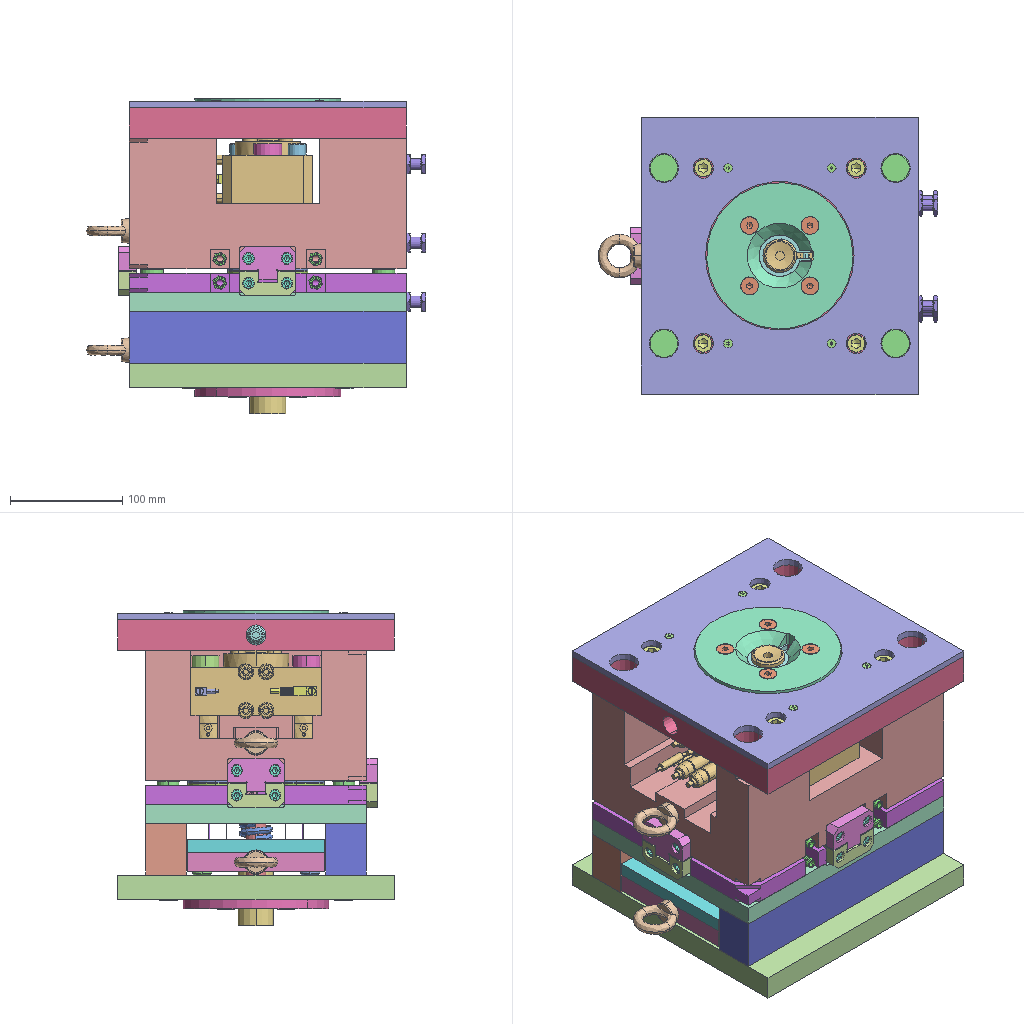Assembly | STEP file | 66 different items | 137 placed | box 302 x 246 x 280 mm
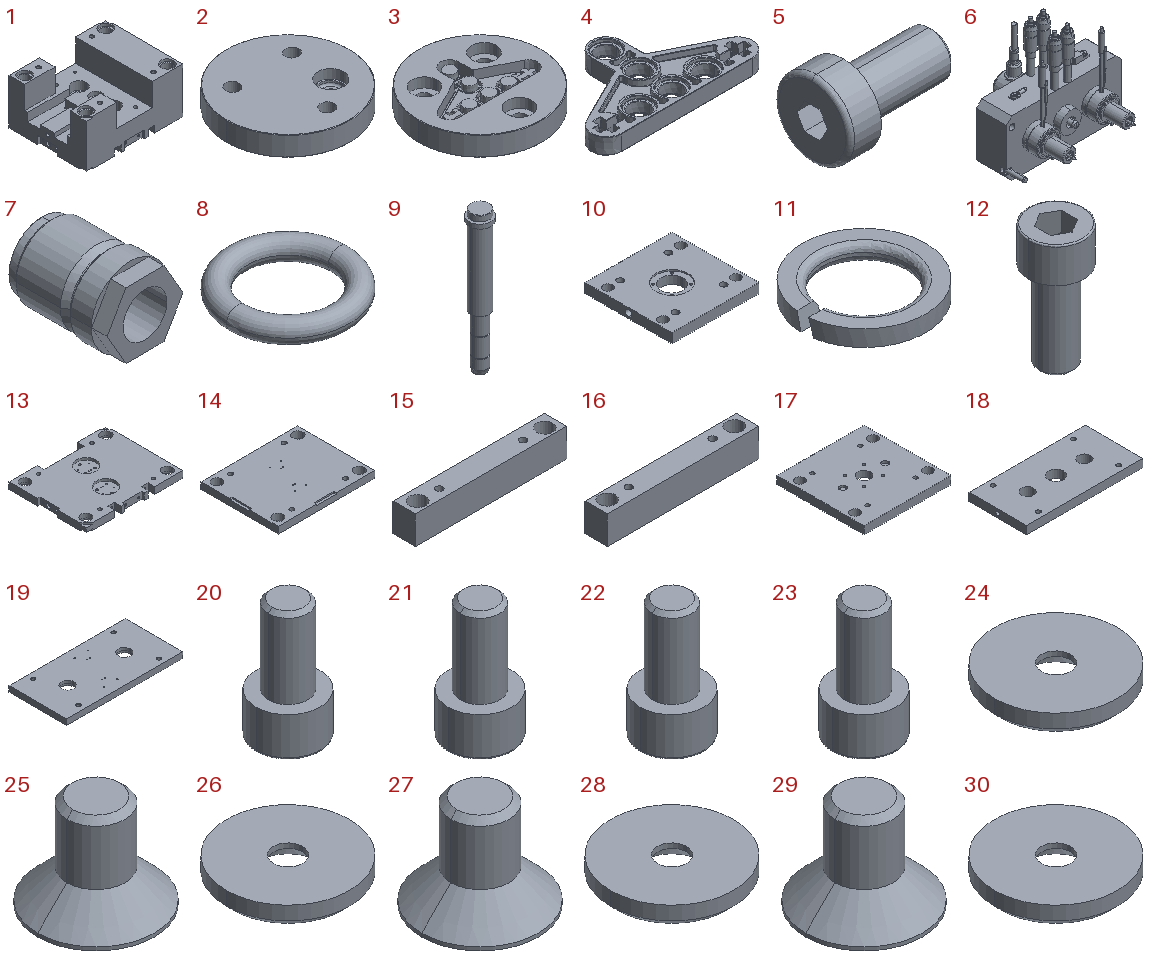Parts list (item | name | quantity | parent item | size | volume):
1 | 2 | x1 | - | 246 x 196 x 116 mm | 3430597 mm3
2 | Cavity | x2 | in Injection system, Forming insert | 50 x 50 x 9.963 mm | 14384 mm3
3 | Core | x2 | in Injection system, Forming insert | 50 x 50 x 8 mm | 13150 mm3
4 | Moulded part | x2 | in Injection system, Forming insert | 39.381 x 23.386 x 3.923 mm | 972.135 mm3
5 | socket head thin cap screw_din_DIN 7984 - M5 x 10 --- 7.6N | x12 | in Injection system, Forming insert | 13.5 x 8.5 x 8.5 mm | 369.151 mm3
6 | COMPANY_A | x1 | in Injection system | - | -
7 | export_nozzle | x2 | in Injection system | 10.5 x 14.1 x 10.5 mm | 682.036 mm3
8 | o-rings_am_J515160x0061H | x2 | in Injection system | 9.3 x 9.3 x 1.6 mm | 48.637 mm3
9 | 38 | x4 | - | 31 x 31 x 200 mm | 90446 mm3
10 | 1 | x1 | - | 246 x 246 x 27 mm | 1437591 mm3
11 | 44 | x4 | - | 15.198 x 15.2 x 2 mm | 183.52 mm3
12 | 45 | x4 | - | 16 x 16 x 35 mm | 3597 mm3
13 | 3 | x1 | in FCPK-196x246_PKA_PKA01-27-1.1730_PKA03-116-1.1730_PKA03-17-1.1730_YES_PKA04-17-1.1730_PKA05-46-1.1730_PKA06-12-1.1730_PKA07-17-1.1730_PKA11-22-1.1730_SLE-75-1.7131_TPE-1.7131 | 246 x 196 x 17 mm | 676741 mm3
14 | 4 | x1 | in FCPK-196x246_PKA_PKA01-27-1.1730_PKA03-116-1.1730_PKA03-17-1.1730_YES_PKA04-17-1.1730_PKA05-46-1.1730_PKA06-12-1.1730_PKA07-17-1.1730_PKA11-22-1.1730_SLE-75-1.7131_TPE-1.7131 | 246 x 196 x 17 mm | 768629 mm3
15 | 5 | x1 | in FCPK-196x246_PKA_PKA01-27-1.1730_PKA03-116-1.1730_PKA03-17-1.1730_YES_PKA04-17-1.1730_PKA05-46-1.1730_PKA06-12-1.1730_PKA07-17-1.1730_PKA11-22-1.1730_SLE-75-1.7131_TPE-1.7131 | 246 x 36 x 46 mm | 349787 mm3
16 | 6 | x1 | in FCPK-196x246_PKA_PKA01-27-1.1730_PKA03-116-1.1730_PKA03-17-1.1730_YES_PKA04-17-1.1730_PKA05-46-1.1730_PKA06-12-1.1730_PKA07-17-1.1730_PKA11-22-1.1730_SLE-75-1.7131_TPE-1.7131 | 246 x 36 x 46 mm | 349787 mm3
17 | 7 | x1 | in FCPK-196x246_PKA_PKA01-27-1.1730_PKA03-116-1.1730_PKA03-17-1.1730_YES_PKA04-17-1.1730_PKA05-46-1.1730_PKA06-12-1.1730_PKA07-17-1.1730_PKA11-22-1.1730_SLE-75-1.7131_TPE-1.7131 | 246 x 246 x 22 mm | 1219815 mm3
18 | 8 | x1 | in FCPK-196x246_PKA_PKA01-27-1.1730_PKA03-116-1.1730_PKA03-17-1.1730_YES_PKA04-17-1.1730_PKA05-46-1.1730_PKA06-12-1.1730_PKA07-17-1.1730_PKA11-22-1.1730_SLE-75-1.7131_TPE-1.7131 | 246 x 122 x 17 mm | 467682 mm3
19 | 9 | x1 | in FCPK-196x246_PKA_PKA01-27-1.1730_PKA03-116-1.1730_PKA03-17-1.1730_YES_PKA04-17-1.1730_PKA05-46-1.1730_PKA06-12-1.1730_PKA07-17-1.1730_PKA11-22-1.1730_SLE-75-1.7131_TPE-1.7131 | 246 x 122 x 12 mm | 330274 mm3
20 | 10 | x1 | in FCPK-196x246_PKA_PKA01-27-1.1730_PKA03-116-1.1730_PKA03-17-1.1730_YES_PKA04-17-1.1730_PKA05-46-1.1730_PKA06-12-1.1730_PKA07-17-1.1730_PKA11-22-1.1730_SLE-75-1.7131_TPE-1.7131 | 13 x 13 x 24 mm | 1690 mm3
21 | 11 | x1 | in FCPK-196x246_PKA_PKA01-27-1.1730_PKA03-116-1.1730_PKA03-17-1.1730_YES_PKA04-17-1.1730_PKA05-46-1.1730_PKA06-12-1.1730_PKA07-17-1.1730_PKA11-22-1.1730_SLE-75-1.7131_TPE-1.7131 | 13 x 13 x 24 mm | 1690 mm3
22 | 12 | x1 | in FCPK-196x246_PKA_PKA01-27-1.1730_PKA03-116-1.1730_PKA03-17-1.1730_YES_PKA04-17-1.1730_PKA05-46-1.1730_PKA06-12-1.1730_PKA07-17-1.1730_PKA11-22-1.1730_SLE-75-1.7131_TPE-1.7131 | 13 x 13 x 24 mm | 1690 mm3
23 | 13 | x1 | in FCPK-196x246_PKA_PKA01-27-1.1730_PKA03-116-1.1730_PKA03-17-1.1730_YES_PKA04-17-1.1730_PKA05-46-1.1730_PKA06-12-1.1730_PKA07-17-1.1730_PKA11-22-1.1730_SLE-75-1.7131_TPE-1.7131 | 13 x 13 x 24 mm | 1690 mm3
24 | 14 | x1 | in FCPK-196x246_PKA_PKA01-27-1.1730_PKA03-116-1.1730_PKA03-17-1.1730_YES_PKA04-17-1.1730_PKA05-46-1.1730_PKA06-12-1.1730_PKA07-17-1.1730_PKA11-22-1.1730_SLE-75-1.7131_TPE-1.7131 | 18 x 18 x 3 mm | 644.142 mm3
25 | 15 | x1 | in FCPK-196x246_PKA_PKA01-27-1.1730_PKA03-116-1.1730_PKA03-17-1.1730_YES_PKA04-17-1.1730_PKA05-46-1.1730_PKA06-12-1.1730_PKA07-17-1.1730_PKA11-22-1.1730_SLE-75-1.7131_TPE-1.7131 | 10 x 10 x 8 mm | 218.465 mm3
26 | 16 | x1 | in FCPK-196x246_PKA_PKA01-27-1.1730_PKA03-116-1.1730_PKA03-17-1.1730_YES_PKA04-17-1.1730_PKA05-46-1.1730_PKA06-12-1.1730_PKA07-17-1.1730_PKA11-22-1.1730_SLE-75-1.7131_TPE-1.7131 | 18 x 18 x 3 mm | 644.142 mm3
27 | 17 | x1 | in FCPK-196x246_PKA_PKA01-27-1.1730_PKA03-116-1.1730_PKA03-17-1.1730_YES_PKA04-17-1.1730_PKA05-46-1.1730_PKA06-12-1.1730_PKA07-17-1.1730_PKA11-22-1.1730_SLE-75-1.7131_TPE-1.7131 | 10 x 10 x 8 mm | 218.465 mm3
28 | 18 | x1 | in FCPK-196x246_PKA_PKA01-27-1.1730_PKA03-116-1.1730_PKA03-17-1.1730_YES_PKA04-17-1.1730_PKA05-46-1.1730_PKA06-12-1.1730_PKA07-17-1.1730_PKA11-22-1.1730_SLE-75-1.7131_TPE-1.7131 | 18 x 18 x 3 mm | 644.142 mm3
29 | 19 | x1 | in FCPK-196x246_PKA_PKA01-27-1.1730_PKA03-116-1.1730_PKA03-17-1.1730_YES_PKA04-17-1.1730_PKA05-46-1.1730_PKA06-12-1.1730_PKA07-17-1.1730_PKA11-22-1.1730_SLE-75-1.7131_TPE-1.7131 | 10 x 10 x 8 mm | 218.465 mm3
30 | 20 | x1 | in FCPK-196x246_PKA_PKA01-27-1.1730_PKA03-116-1.1730_PKA03-17-1.1730_YES_PKA04-17-1.1730_PKA05-46-1.1730_PKA06-12-1.1730_PKA07-17-1.1730_PKA11-22-1.1730_SLE-75-1.7131_TPE-1.7131 | 18 x 18 x 3 mm | 644.142 mm3
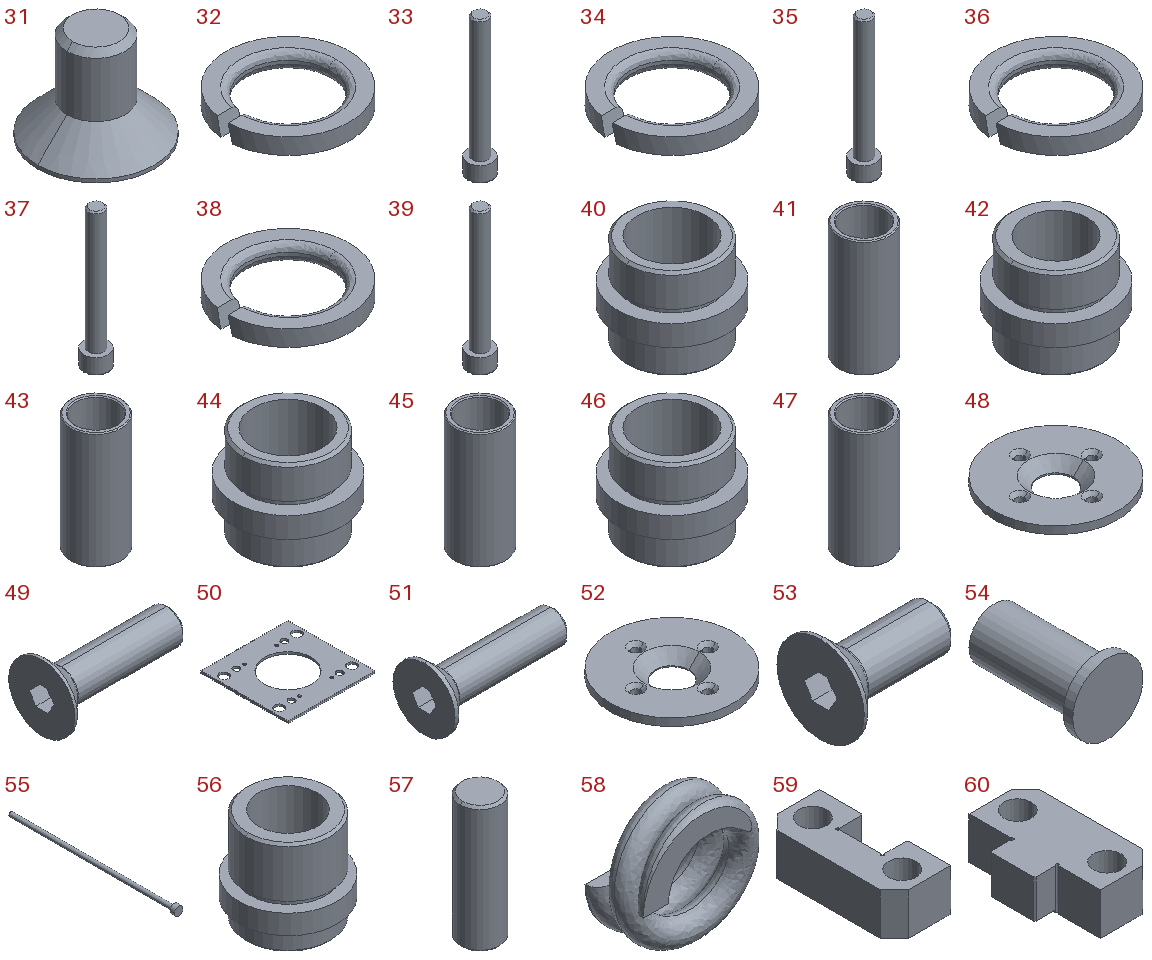31 | 21 | x1 | in FCPK-196x246_PKA_PKA01-27-1.1730_PKA03-116-1.1730_PKA03-17-1.1730_YES_PKA04-17-1.1730_PKA05-46-1.1730_PKA06-12-1.1730_PKA07-17-1.1730_PKA11-22-1.1730_SLE-75-1.7131_TPE-1.7131 | 10 x 10 x 8 mm | 218.465 mm3
32 | 22 | x1 | in FCPK-196x246_PKA_PKA01-27-1.1730_PKA03-116-1.1730_PKA03-17-1.1730_YES_PKA04-17-1.1730_PKA05-46-1.1730_PKA06-12-1.1730_PKA07-17-1.1730_PKA11-22-1.1730_SLE-75-1.7131_TPE-1.7131 | 15.198 x 15.2 x 2 mm | 183.545 mm3
33 | 23 | x1 | in FCPK-196x246_PKA_PKA01-27-1.1730_PKA03-116-1.1730_PKA03-17-1.1730_YES_PKA04-17-1.1730_PKA05-46-1.1730_PKA06-12-1.1730_PKA07-17-1.1730_PKA11-22-1.1730_SLE-75-1.7131_TPE-1.7131 | 16 x 16 x 90 mm | 7916 mm3
34 | 24 | x1 | in FCPK-196x246_PKA_PKA01-27-1.1730_PKA03-116-1.1730_PKA03-17-1.1730_YES_PKA04-17-1.1730_PKA05-46-1.1730_PKA06-12-1.1730_PKA07-17-1.1730_PKA11-22-1.1730_SLE-75-1.7131_TPE-1.7131 | 15.198 x 15.2 x 2 mm | 183.545 mm3
35 | 25 | x1 | in FCPK-196x246_PKA_PKA01-27-1.1730_PKA03-116-1.1730_PKA03-17-1.1730_YES_PKA04-17-1.1730_PKA05-46-1.1730_PKA06-12-1.1730_PKA07-17-1.1730_PKA11-22-1.1730_SLE-75-1.7131_TPE-1.7131 | 16 x 16 x 90 mm | 7916 mm3
36 | 26 | x1 | in FCPK-196x246_PKA_PKA01-27-1.1730_PKA03-116-1.1730_PKA03-17-1.1730_YES_PKA04-17-1.1730_PKA05-46-1.1730_PKA06-12-1.1730_PKA07-17-1.1730_PKA11-22-1.1730_SLE-75-1.7131_TPE-1.7131 | 15.198 x 15.2 x 2 mm | 183.545 mm3
37 | 27 | x1 | in FCPK-196x246_PKA_PKA01-27-1.1730_PKA03-116-1.1730_PKA03-17-1.1730_YES_PKA04-17-1.1730_PKA05-46-1.1730_PKA06-12-1.1730_PKA07-17-1.1730_PKA11-22-1.1730_SLE-75-1.7131_TPE-1.7131 | 16 x 16 x 90 mm | 7916 mm3
38 | 28 | x1 | in FCPK-196x246_PKA_PKA01-27-1.1730_PKA03-116-1.1730_PKA03-17-1.1730_YES_PKA04-17-1.1730_PKA05-46-1.1730_PKA06-12-1.1730_PKA07-17-1.1730_PKA11-22-1.1730_SLE-75-1.7131_TPE-1.7131 | 15.198 x 15.2 x 2 mm | 183.545 mm3
39 | 29 | x1 | in FCPK-196x246_PKA_PKA01-27-1.1730_PKA03-116-1.1730_PKA03-17-1.1730_YES_PKA04-17-1.1730_PKA05-46-1.1730_PKA06-12-1.1730_PKA07-17-1.1730_PKA11-22-1.1730_SLE-75-1.7131_TPE-1.7131 | 16 x 16 x 90 mm | 7916 mm3
40 | 30 | x1 | in FCPK-196x246_PKA_PKA01-27-1.1730_PKA03-116-1.1730_PKA03-17-1.1730_YES_PKA04-17-1.1730_PKA05-46-1.1730_PKA06-12-1.1730_PKA07-17-1.1730_PKA11-22-1.1730_SLE-75-1.7131_TPE-1.7131 | 31 x 31 x 26 mm | 6604 mm3
41 | 31 | x1 | in FCPK-196x246_PKA_PKA01-27-1.1730_PKA03-116-1.1730_PKA03-17-1.1730_YES_PKA04-17-1.1730_PKA05-46-1.1730_PKA06-12-1.1730_PKA07-17-1.1730_PKA11-22-1.1730_SLE-75-1.7131_TPE-1.7131 | 26 x 26 x 60 mm | 14379 mm3
42 | 32 | x1 | in FCPK-196x246_PKA_PKA01-27-1.1730_PKA03-116-1.1730_PKA03-17-1.1730_YES_PKA04-17-1.1730_PKA05-46-1.1730_PKA06-12-1.1730_PKA07-17-1.1730_PKA11-22-1.1730_SLE-75-1.7131_TPE-1.7131 | 31 x 31 x 26 mm | 8159 mm3
43 | 33 | x1 | in FCPK-196x246_PKA_PKA01-27-1.1730_PKA03-116-1.1730_PKA03-17-1.1730_YES_PKA04-17-1.1730_PKA05-46-1.1730_PKA06-12-1.1730_PKA07-17-1.1730_PKA11-22-1.1730_SLE-75-1.7131_TPE-1.7131 | 26 x 26 x 60 mm | 14379 mm3
44 | 34 | x1 | in FCPK-196x246_PKA_PKA01-27-1.1730_PKA03-116-1.1730_PKA03-17-1.1730_YES_PKA04-17-1.1730_PKA05-46-1.1730_PKA06-12-1.1730_PKA07-17-1.1730_PKA11-22-1.1730_SLE-75-1.7131_TPE-1.7131 | 31 x 31 x 26 mm | 6604 mm3
45 | 35 | x1 | in FCPK-196x246_PKA_PKA01-27-1.1730_PKA03-116-1.1730_PKA03-17-1.1730_YES_PKA04-17-1.1730_PKA05-46-1.1730_PKA06-12-1.1730_PKA07-17-1.1730_PKA11-22-1.1730_SLE-75-1.7131_TPE-1.7131 | 26 x 26 x 60 mm | 14379 mm3
46 | 36 | x1 | in FCPK-196x246_PKA_PKA01-27-1.1730_PKA03-116-1.1730_PKA03-17-1.1730_YES_PKA04-17-1.1730_PKA05-46-1.1730_PKA06-12-1.1730_PKA07-17-1.1730_PKA11-22-1.1730_SLE-75-1.7131_TPE-1.7131 | 31 x 31 x 26 mm | 6604 mm3
47 | 37 | x1 | in FCPK-196x246_PKA_PKA01-27-1.1730_PKA03-116-1.1730_PKA03-17-1.1730_YES_PKA04-17-1.1730_PKA05-46-1.1730_PKA06-12-1.1730_PKA07-17-1.1730_PKA11-22-1.1730_SLE-75-1.7131_TPE-1.7131 | 26 x 26 x 60 mm | 14379 mm3
48 | PCA-130120 | x1 | - | 130 x 130 x 12 mm | 106365 mm3
49 | socket countersunk head screw_din_DIN 7991 - M8 x 30 --- 21.8N | x4 | - | 30 x 15.57 x 15.57 mm | 1740 mm3
50 | Insulating plate | x2 | - | 246 x 246 x 6 mm | 261647 mm3
51 | socket countersunk head screw_din_DIN 7991 - M4 x 16 --- 11.6N | x4 | - | 16 x 7.64 x 7.64 mm | 232.169 mm3
52 | PCA-130120 unmachined | x1 | - | 130 x 130 x 12 mm | 107256 mm3
53 | socket countersunk head screw_din_DIN 7991 - M8 x 20 --- 11.8N | x4 | - | 20 x 15.57 x 15.57 mm | 1237 mm3
54 | Main ejector | x1 | - | 44 x 71 x 44 mm | 61399 mm3
55 | ejector | x8 | - | 3 x 58.08 x 3 mm | 97.701 mm3
56 | TBW-1812 | x2 | - | 30 x 30 x 29 mm | 8727 mm3
57 | Ejector guide | x2 | - | 18 x 18 x 58 mm | 14705 mm3
58 | Ejector spring 14 | x2 | - | 30 x 14 x 30 mm | 3867 mm3
59 | 1_1 | x2 | in MS50-050 | 21.5 x 50 x 16 mm | 12210 mm3
60 | 2_1 | x2 | in MS50-050 | 30 x 50 x 16 mm | 16891 mm3
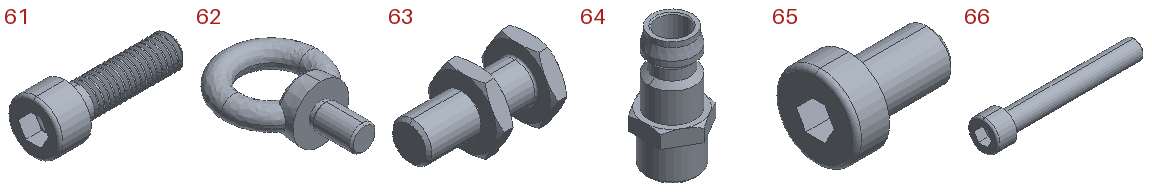61 | socket head cap screw 4762_din_ISO 4762 M6 x 20 --- 20S | x8 | in MS50-050 | 26 x 10 x 10 mm | 892.13 mm3
62 | Part 65 | x2 | - | 38.75 x 55.625 x 21.875 mm | 8627 mm3
63 | Part 66 | x6 | - | 31.25 x 19.486 x 16.875 mm | 3681 mm3
64 | KH-060 ENM 10 | x8 | - | 11 x 12.702 x 24 mm | 962.573 mm3
65 | socket head thin cap screw_din_DIN 7984 - M6 x 10 --- 7N | x4 | - | 14 x 10 x 10 mm | 545.673 mm3
66 | socket head cap screw fine_din_DIN 912 M10x1 x 70 --- 32N | x2 | - | 80 x 16 x 16 mm | 7176 mm3
Placements (level | parent | child | x y z in mm | rotation matrix by rows):
1 | subassembly 2 | 2 | -0.0 -0.0 -0.0 | 1 0 0 0 1 0 0 0 1
1 | subassembly 2 | Injection system | 52.614 -35.372 53.014 | 1 0 0 0 1 0 0 0 1
2 | Injection system | Cavity | -79.114 -4.052 45.024 | 1 0 0 0 1 0 0 0 1
2 | Injection system | Core | -79.114 -4.052 45.024 | 1 0 0 0 1 0 0 0 1
2 | Injection system | Moulded part | -79.114 -4.052 45.024 | 1 0 0 0 1 0 0 0 1
2 | Injection system | socket head thin cap screw_din_DIN 7984 - M5 x 10 --- 7.6N | -51.122 10.1 46.586 | 0 0 1 0 1 0 -1 0 0
2 | Injection system | socket head thin cap screw_din_DIN 7984 - M5 x 10 --- 7.6N | -63.214 -16.378 47.386 | 0 -0.383 -0.9237 0 0.9237 -0.383 1 0 0
2 | Injection system | socket head thin cap screw_din_DIN 7984 - M5 x 10 --- 7.6N | -63.214 -16.378 46.586 | 0 0 1 0 1 0 -1 0 0
2 | Injection system | socket head thin cap screw_din_DIN 7984 - M5 x 10 --- 7.6N | -75.306 10.1 46.586 | 0 0 1 0 1 0 -1 0 0
2 | Injection system | socket head thin cap screw_din_DIN 7984 - M5 x 10 --- 7.6N | -75.306 10.1 47.386 | 0 -0.383 -0.9237 0 0.9237 -0.383 1 0 0
2 | Injection system | socket head thin cap screw_din_DIN 7984 - M5 x 10 --- 7.6N | -51.122 10.1 47.386 | 0 -0.383 -0.9237 0 0.9237 -0.383 1 0 0
2 | Injection system | COMPANY_A | -52.614 35.372 149.986 | 0 0 -1 -1 0 0 0 1 0
2 | Injection system | Forming insert | -105.228 70.745 0.0 | -1 0 0 0 -1 0 0 0 1
3 | Forming insert | Cavity | -79.114 -4.052 45.024 | 1 0 0 0 1 0 0 0 1
3 | Forming insert | Core | -79.114 -4.052 45.024 | 1 0 0 0 1 0 0 0 1
3 | Forming insert | Moulded part | -79.114 -4.052 45.024 | 1 0 0 0 1 0 0 0 1
3 | Forming insert | socket head thin cap screw_din_DIN 7984 - M5 x 10 --- 7.6N | -51.122 10.1 46.586 | 0 0 1 0 1 0 -1 0 0
3 | Forming insert | socket head thin cap screw_din_DIN 7984 - M5 x 10 --- 7.6N | -63.214 -16.378 47.386 | 0 -0.383 -0.9237 0 0.9237 -0.383 1 0 0
3 | Forming insert | socket head thin cap screw_din_DIN 7984 - M5 x 10 --- 7.6N | -63.214 -16.378 46.586 | 0 0 1 0 1 0 -1 0 0
3 | Forming insert | socket head thin cap screw_din_DIN 7984 - M5 x 10 --- 7.6N | -75.306 10.1 46.586 | 0 0 1 0 1 0 -1 0 0
3 | Forming insert | socket head thin cap screw_din_DIN 7984 - M5 x 10 --- 7.6N | -75.306 10.1 47.386 | 0 -0.383 -0.9237 0 0.9237 -0.383 1 0 0
3 | Forming insert | socket head thin cap screw_din_DIN 7984 - M5 x 10 --- 7.6N | -51.122 10.1 47.386 | 0 -0.383 -0.9237 0 0.9237 -0.383 1 0 0
2 | Injection system | export_nozzle | -10.114 -7.128 146.986 | 1 0 0 0 0 -1 0 1 0
2 | Injection system | export_nozzle | -10.114 77.872 146.986 | 1 0 0 0 0 -1 0 1 0
2 | Injection system | o-rings_am_J515160x0061H | -52.614 77.872 50.486 | 1 0 0 0 1 0 0 0 1
2 | Injection system | o-rings_am_J515160x0061H | -52.614 -7.128 50.486 | -0.9237 -0.383 0 -0.383 0.9237 0 0 0 -1
1 | subassembly 2 | 38 | -0.0 -156.0 -0.0 | 1 0 0 0 1 0 0 0 1
1 | subassembly 2 | 1 | -0.0 -0.0 -0.0 | 1 0 0 0 1 0 0 0 1
1 | subassembly 2 | 44 | -136.0 -156.0 -0.0 | 1 0 0 0 1 0 0 0 1
1 | subassembly 2 | 45 | -136.0 -156.0 0.0 | 1 0 0 0 1 0 0 0 1
1 | subassembly 2 | 38 | -206.0 156.0 -0.0 | -1 0 0 0 -1 0 0 0 1
1 | subassembly 2 | 45 | -0.0 156.0 0.0 | -1 0 0 0 -1 0 0 0 1
1 | subassembly 2 | 44 | -136.0 -0.0 -0.0 | 1 0 0 0 1 0 0 0 1
1 | subassembly 2 | 38 | 206.0 -156.0 -0.0 | 1 0 0 0 1 0 0 0 1
1 | subassembly 2 | 45 | -0.0 -156.0 0.0 | 1 0 0 0 1 0 0 0 1
1 | subassembly 2 | 44 | 136.0 -0.0 -0.0 | -1 0 0 0 -1 0 0 0 1
1 | subassembly 2 | 38 | -0.0 156.0 -0.0 | -1 0 0 0 -1 0 0 0 1
1 | subassembly 2 | 45 | 136.0 156.0 0.0 | -1 0 0 0 -1 0 0 0 1
1 | subassembly 2 | 44 | 136.0 156.0 -0.0 | -1 0 0 0 -1 0 0 0 1
1 | subassembly 2 | FCPK-196x246_PKA_PKA01-27-1.173_PKA03-116-1.173_PKA03-17-1.173_YES_PKA04-17-1.173_PKA05-46-1.173_PKA06-12-1.173_PKA07-17-1.173_PKA11-22-1.173_SLE-75-1.713_TPE-1.713 | 0.0 -0.0 -4.0 | 1 0 0 0 1 0 0 0 1
2 | FCPK-196x246_PKA_PKA01-27-1.173_PKA03-116-1.173_PKA03-17-1.173_YES_PKA04-17-1.173_PKA05-46-1.173_PKA06-12-1.173_PKA07-17-1.173_PKA11-22-1.173_SLE-75-1.713_TPE-1.713 | 3 | -0.0 -0.0 -0.0 | 1 0 0 0 1 0 0 0 1
2 | FCPK-196x246_PKA_PKA01-27-1.173_PKA03-116-1.173_PKA03-17-1.173_YES_PKA04-17-1.173_PKA05-46-1.173_PKA06-12-1.173_PKA07-17-1.173_PKA11-22-1.173_SLE-75-1.713_TPE-1.713 | 4 | -0.0 -0.0 -0.0 | 1 0 0 0 1 0 0 0 1
2 | FCPK-196x246_PKA_PKA01-27-1.173_PKA03-116-1.173_PKA03-17-1.173_YES_PKA04-17-1.173_PKA05-46-1.173_PKA06-12-1.173_PKA07-17-1.173_PKA11-22-1.173_SLE-75-1.713_TPE-1.713 | 5 | -0.0 -0.0 -0.0 | 1 0 0 0 1 0 0 0 1
2 | FCPK-196x246_PKA_PKA01-27-1.173_PKA03-116-1.173_PKA03-17-1.173_YES_PKA04-17-1.173_PKA05-46-1.173_PKA06-12-1.173_PKA07-17-1.173_PKA11-22-1.173_SLE-75-1.713_TPE-1.713 | 6 | -0.0 -0.0 -0.0 | 1 0 0 0 1 0 0 0 1
2 | FCPK-196x246_PKA_PKA01-27-1.173_PKA03-116-1.173_PKA03-17-1.173_YES_PKA04-17-1.173_PKA05-46-1.173_PKA06-12-1.173_PKA07-17-1.173_PKA11-22-1.173_SLE-75-1.713_TPE-1.713 | 7 | -0.0 -0.0 -0.0 | 1 0 0 0 1 0 0 0 1
2 | FCPK-196x246_PKA_PKA01-27-1.173_PKA03-116-1.173_PKA03-17-1.173_YES_PKA04-17-1.173_PKA05-46-1.173_PKA06-12-1.173_PKA07-17-1.173_PKA11-22-1.173_SLE-75-1.713_TPE-1.713 | 8 | -0.0 -0.0 -0.0 | 1 0 0 0 1 0 0 0 1
2 | FCPK-196x246_PKA_PKA01-27-1.173_PKA03-116-1.173_PKA03-17-1.173_YES_PKA04-17-1.173_PKA05-46-1.173_PKA06-12-1.173_PKA07-17-1.173_PKA11-22-1.173_SLE-75-1.713_TPE-1.713 | 9 | -0.0 -0.0 -0.0 | 1 0 0 0 1 0 0 0 1
2 | FCPK-196x246_PKA_PKA01-27-1.173_PKA03-116-1.173_PKA03-17-1.173_YES_PKA04-17-1.173_PKA05-46-1.173_PKA06-12-1.173_PKA07-17-1.173_PKA11-22-1.173_SLE-75-1.713_TPE-1.713 | 10 | -0.0 -0.0 -0.0 | 1 0 0 0 1 0 0 0 1
2 | FCPK-196x246_PKA_PKA01-27-1.173_PKA03-116-1.173_PKA03-17-1.173_YES_PKA04-17-1.173_PKA05-46-1.173_PKA06-12-1.173_PKA07-17-1.173_PKA11-22-1.173_SLE-75-1.713_TPE-1.713 | 11 | -0.0 -0.0 -0.0 | 1 0 0 0 1 0 0 0 1
2 | FCPK-196x246_PKA_PKA01-27-1.173_PKA03-116-1.173_PKA03-17-1.173_YES_PKA04-17-1.173_PKA05-46-1.173_PKA06-12-1.173_PKA07-17-1.173_PKA11-22-1.173_SLE-75-1.713_TPE-1.713 | 12 | -0.0 -0.0 -0.0 | 1 0 0 0 1 0 0 0 1
2 | FCPK-196x246_PKA_PKA01-27-1.173_PKA03-116-1.173_PKA03-17-1.173_YES_PKA04-17-1.173_PKA05-46-1.173_PKA06-12-1.173_PKA07-17-1.173_PKA11-22-1.173_SLE-75-1.713_TPE-1.713 | 13 | -0.0 -0.0 -0.0 | 1 0 0 0 1 0 0 0 1
2 | FCPK-196x246_PKA_PKA01-27-1.173_PKA03-116-1.173_PKA03-17-1.173_YES_PKA04-17-1.173_PKA05-46-1.173_PKA06-12-1.173_PKA07-17-1.173_PKA11-22-1.173_SLE-75-1.713_TPE-1.713 | 14 | -0.0 -0.0 -0.0 | 1 0 0 0 1 0 0 0 1
2 | FCPK-196x246_PKA_PKA01-27-1.173_PKA03-116-1.173_PKA03-17-1.173_YES_PKA04-17-1.173_PKA05-46-1.173_PKA06-12-1.173_PKA07-17-1.173_PKA11-22-1.173_SLE-75-1.713_TPE-1.713 | 15 | -0.0 -0.0 -0.0 | 1 0 0 0 1 0 0 0 1
2 | FCPK-196x246_PKA_PKA01-27-1.173_PKA03-116-1.173_PKA03-17-1.173_YES_PKA04-17-1.173_PKA05-46-1.173_PKA06-12-1.173_PKA07-17-1.173_PKA11-22-1.173_SLE-75-1.713_TPE-1.713 | 16 | -0.0 -0.0 -0.0 | 1 0 0 0 1 0 0 0 1
2 | FCPK-196x246_PKA_PKA01-27-1.173_PKA03-116-1.173_PKA03-17-1.173_YES_PKA04-17-1.173_PKA05-46-1.173_PKA06-12-1.173_PKA07-17-1.173_PKA11-22-1.173_SLE-75-1.713_TPE-1.713 | 17 | -0.0 -0.0 -0.0 | 1 0 0 0 1 0 0 0 1
2 | FCPK-196x246_PKA_PKA01-27-1.173_PKA03-116-1.173_PKA03-17-1.173_YES_PKA04-17-1.173_PKA05-46-1.173_PKA06-12-1.173_PKA07-17-1.173_PKA11-22-1.173_SLE-75-1.713_TPE-1.713 | 18 | -0.0 -0.0 -0.0 | 1 0 0 0 1 0 0 0 1
2 | FCPK-196x246_PKA_PKA01-27-1.173_PKA03-116-1.173_PKA03-17-1.173_YES_PKA04-17-1.173_PKA05-46-1.173_PKA06-12-1.173_PKA07-17-1.173_PKA11-22-1.173_SLE-75-1.713_TPE-1.713 | 19 | -0.0 -0.0 -0.0 | 1 0 0 0 1 0 0 0 1
2 | FCPK-196x246_PKA_PKA01-27-1.173_PKA03-116-1.173_PKA03-17-1.173_YES_PKA04-17-1.173_PKA05-46-1.173_PKA06-12-1.173_PKA07-17-1.173_PKA11-22-1.173_SLE-75-1.713_TPE-1.713 | 20 | -0.0 -0.0 -0.0 | 1 0 0 0 1 0 0 0 1
2 | FCPK-196x246_PKA_PKA01-27-1.173_PKA03-116-1.173_PKA03-17-1.173_YES_PKA04-17-1.173_PKA05-46-1.173_PKA06-12-1.173_PKA07-17-1.173_PKA11-22-1.173_SLE-75-1.713_TPE-1.713 | 21 | -0.0 -0.0 -0.0 | 1 0 0 0 1 0 0 0 1
2 | FCPK-196x246_PKA_PKA01-27-1.173_PKA03-116-1.173_PKA03-17-1.173_YES_PKA04-17-1.173_PKA05-46-1.173_PKA06-12-1.173_PKA07-17-1.173_PKA11-22-1.173_SLE-75-1.713_TPE-1.713 | 22 | -0.0 -0.0 -0.0 | 1 0 0 0 1 0 0 0 1
2 | FCPK-196x246_PKA_PKA01-27-1.173_PKA03-116-1.173_PKA03-17-1.173_YES_PKA04-17-1.173_PKA05-46-1.173_PKA06-12-1.173_PKA07-17-1.173_PKA11-22-1.173_SLE-75-1.713_TPE-1.713 | 23 | -0.0 -0.0 -0.0 | 1 0 0 0 1 0 0 0 1
2 | FCPK-196x246_PKA_PKA01-27-1.173_PKA03-116-1.173_PKA03-17-1.173_YES_PKA04-17-1.173_PKA05-46-1.173_PKA06-12-1.173_PKA07-17-1.173_PKA11-22-1.173_SLE-75-1.713_TPE-1.713 | 24 | -0.0 -0.0 -0.0 | 1 0 0 0 1 0 0 0 1
2 | FCPK-196x246_PKA_PKA01-27-1.173_PKA03-116-1.173_PKA03-17-1.173_YES_PKA04-17-1.173_PKA05-46-1.173_PKA06-12-1.173_PKA07-17-1.173_PKA11-22-1.173_SLE-75-1.713_TPE-1.713 | 25 | -0.0 -0.0 -0.0 | 1 0 0 0 1 0 0 0 1
2 | FCPK-196x246_PKA_PKA01-27-1.173_PKA03-116-1.173_PKA03-17-1.173_YES_PKA04-17-1.173_PKA05-46-1.173_PKA06-12-1.173_PKA07-17-1.173_PKA11-22-1.173_SLE-75-1.713_TPE-1.713 | 26 | -0.0 -0.0 -0.0 | 1 0 0 0 1 0 0 0 1
2 | FCPK-196x246_PKA_PKA01-27-1.173_PKA03-116-1.173_PKA03-17-1.173_YES_PKA04-17-1.173_PKA05-46-1.173_PKA06-12-1.173_PKA07-17-1.173_PKA11-22-1.173_SLE-75-1.713_TPE-1.713 | 27 | -0.0 -0.0 -0.0 | 1 0 0 0 1 0 0 0 1
2 | FCPK-196x246_PKA_PKA01-27-1.173_PKA03-116-1.173_PKA03-17-1.173_YES_PKA04-17-1.173_PKA05-46-1.173_PKA06-12-1.173_PKA07-17-1.173_PKA11-22-1.173_SLE-75-1.713_TPE-1.713 | 28 | -0.0 -0.0 -0.0 | 1 0 0 0 1 0 0 0 1
2 | FCPK-196x246_PKA_PKA01-27-1.173_PKA03-116-1.173_PKA03-17-1.173_YES_PKA04-17-1.173_PKA05-46-1.173_PKA06-12-1.173_PKA07-17-1.173_PKA11-22-1.173_SLE-75-1.713_TPE-1.713 | 29 | -0.0 -0.0 -0.0 | 1 0 0 0 1 0 0 0 1
2 | FCPK-196x246_PKA_PKA01-27-1.173_PKA03-116-1.173_PKA03-17-1.173_YES_PKA04-17-1.173_PKA05-46-1.173_PKA06-12-1.173_PKA07-17-1.173_PKA11-22-1.173_SLE-75-1.713_TPE-1.713 | 30 | -0.0 -0.0 -0.0 | 1 0 0 0 1 0 0 0 1
2 | FCPK-196x246_PKA_PKA01-27-1.173_PKA03-116-1.173_PKA03-17-1.173_YES_PKA04-17-1.173_PKA05-46-1.173_PKA06-12-1.173_PKA07-17-1.173_PKA11-22-1.173_SLE-75-1.713_TPE-1.713 | 31 | -0.0 -0.0 -0.0 | 1 0 0 0 1 0 0 0 1
2 | FCPK-196x246_PKA_PKA01-27-1.173_PKA03-116-1.173_PKA03-17-1.173_YES_PKA04-17-1.173_PKA05-46-1.173_PKA06-12-1.173_PKA07-17-1.173_PKA11-22-1.173_SLE-75-1.713_TPE-1.713 | 32 | -0.0 -0.0 -0.0 | 1 0 0 0 1 0 0 0 1
2 | FCPK-196x246_PKA_PKA01-27-1.173_PKA03-116-1.173_PKA03-17-1.173_YES_PKA04-17-1.173_PKA05-46-1.173_PKA06-12-1.173_PKA07-17-1.173_PKA11-22-1.173_SLE-75-1.713_TPE-1.713 | 33 | -0.0 -0.0 -0.0 | 1 0 0 0 1 0 0 0 1
2 | FCPK-196x246_PKA_PKA01-27-1.173_PKA03-116-1.173_PKA03-17-1.173_YES_PKA04-17-1.173_PKA05-46-1.173_PKA06-12-1.173_PKA07-17-1.173_PKA11-22-1.173_SLE-75-1.713_TPE-1.713 | 34 | -0.0 -0.0 -0.0 | 1 0 0 0 1 0 0 0 1
2 | FCPK-196x246_PKA_PKA01-27-1.173_PKA03-116-1.173_PKA03-17-1.173_YES_PKA04-17-1.173_PKA05-46-1.173_PKA06-12-1.173_PKA07-17-1.173_PKA11-22-1.173_SLE-75-1.713_TPE-1.713 | 35 | -0.0 -0.0 -0.0 | 1 0 0 0 1 0 0 0 1
2 | FCPK-196x246_PKA_PKA01-27-1.173_PKA03-116-1.173_PKA03-17-1.173_YES_PKA04-17-1.173_PKA05-46-1.173_PKA06-12-1.173_PKA07-17-1.173_PKA11-22-1.173_SLE-75-1.713_TPE-1.713 | 36 | -0.0 -0.0 -0.0 | 1 0 0 0 1 0 0 0 1
2 | FCPK-196x246_PKA_PKA01-27-1.173_PKA03-116-1.173_PKA03-17-1.173_YES_PKA04-17-1.173_PKA05-46-1.173_PKA06-12-1.173_PKA07-17-1.173_PKA11-22-1.173_SLE-75-1.713_TPE-1.713 | 37 | -0.0 -0.0 -0.0 | 1 0 0 0 1 0 0 0 1
1 | subassembly 2 | PCA-130120 | 0.0 0.0 241.0 | -0.7071 -0.7071 0 0.7071 -0.7071 0 0 0 1
1 | subassembly 2 | socket countersunk head screw_din_DIN 7991 - M8 x 30 --- 21.8N | -26.87 -26.87 253.4 | 0 0 1 0 1 0 -1 0 0
1 | subassembly 2 | socket countersunk head screw_din_DIN 7991 - M8 x 30 --- 21.8N | 26.87 -26.87 253.4 | 0 -1 0 0 0 1 -1 0 0
1 | subassembly 2 | socket countersunk head screw_din_DIN 7991 - M8 x 30 --- 21.8N | 26.87 26.87 253.4 | 0 0 -1 0 -1 0 -1 0 0
1 | subassembly 2 | socket countersunk head screw_din_DIN 7991 - M8 x 30 --- 21.8N | -26.87 26.87 253.4 | 0 1 0 0 0 -1 -1 0 0
1 | subassembly 2 | Insulating plate | 0.0 0.0 245.0 | 1 0 0 0 1 0 0 0 1
1 | subassembly 2 | socket countersunk head screw_din_DIN 7991 - M4 x 16 --- 11.6N | -46.0 -78.0 251.3 | 0 0 1 0 1 0 -1 0 0
1 | subassembly 2 | socket countersunk head screw_din_DIN 7991 - M4 x 16 --- 11.6N | -46.0 78.0 251.3 | 0 0 -1 0 -1 0 -1 0 0
1 | subassembly 2 | socket countersunk head screw_din_DIN 7991 - M4 x 16 --- 11.6N | 46.0 78.0 251.3 | 0 0 -1 0 -1 0 -1 0 0
1 | subassembly 2 | Insulating plate | 0.0 0.0 245.0 | 1 0 0 0 1 0 0 0 1
1 | subassembly 2 | socket countersunk head screw_din_DIN 7991 - M4 x 16 --- 11.6N | 46.0 -78.0 251.3 | 0 0 1 0 1 0 -1 0 0
1 | subassembly 2 | PCA-130120 unmachined | -0.0 -0.0 -0.0 | -0.7071 -0.7071 0 -0.7071 0.7071 0 0 0 -1
1 | subassembly 2 | socket countersunk head screw_din_DIN 7991 - M8 x 20 --- 11.8N | -26.87 -26.87 -12.4 | 0 -0.383 -0.9237 0 0.9237 -0.383 1 0 0
1 | subassembly 2 | socket countersunk head screw_din_DIN 7991 - M8 x 20 --- 11.8N | 26.87 -26.87 -12.4 | 0 -0.9237 0.383 0 -0.383 -0.9237 1 0 0
1 | subassembly 2 | socket countersunk head screw_din_DIN 7991 - M8 x 20 --- 11.8N | 26.87 26.87 -12.4 | 0 0.383 0.9237 0 -0.9237 0.383 1 0 0
1 | subassembly 2 | socket countersunk head screw_din_DIN 7991 - M8 x 20 --- 11.8N | -26.87 26.87 -12.4 | 0 0.9237 -0.383 0 0.383 0.9237 1 0 0
1 | subassembly 2 | Main ejector | 0.0 0.0 44.0 | 1 0 0 0 0 1 0 -1 0
1 | subassembly 2 | ejector | 13.436 26.121 38.0 | 1 0 0 0 0 -1 0 1 0
1 | subassembly 2 | ejector | 24.5 41.882 38.0 | 1 0 0 0 0 -1 0 1 0
1 | subassembly 2 | ejector | -3.3 41.882 38.0 | 1 0 0 0 0 -1 0 1 0
1 | subassembly 2 | ejector | -7.764 -26.121 38.0 | 1 0 0 0 0 -1 0 1 0
1 | subassembly 2 | ejector | 3.3 -41.882 38.0 | 1 0 0 0 0 -1 0 1 0
1 | subassembly 2 | ejector | -24.5 -41.882 38.0 | 1 0 0 0 0 -1 0 1 0
1 | subassembly 2 | ejector | 7.764 26.121 38.0 | 1 0 0 0 0 -1 0 1 0
1 | subassembly 2 | ejector | -13.436 -26.121 38.0 | 1 0 0 0 0 -1 0 1 0
1 | subassembly 2 | TBW-1812 | 60.0 0.0 50.0 | -0.9237 -0.383 0 -0.383 0.9237 0 0 0 -1
1 | subassembly 2 | TBW-1812 | -60.0 0.0 50.0 | -0.9237 -0.383 0 -0.383 0.9237 0 0 0 -1
1 | subassembly 2 | Ejector guide | -60.0 0.0 12.0 | 1 0 0 0 1 0 0 0 1
1 | subassembly 2 | Ejector guide | 60.0 0.0 12.0 | 1 0 0 0 1 0 0 0 1
1 | subassembly 2 | Ejector spring 14 | 60.0 0.0 64.0 | 1 0 0 0 0 1 0 -1 0
1 | subassembly 2 | Ejector spring 14 | -60.0 0.0 64.0 | 1 0 0 0 0 1 0 -1 0
1 | subassembly 2 | MS50-050 | -117.0 25.0 78.0 | 0 1 0 -1 0 0 0 0 1
2 | MS50-050 | 1_1 | 25.0 0.0 21.5 | 0 -1 0 0 0 -1 1 0 0
2 | MS50-050 | 2_1 | 25.0 -0.0 22.5 | 0 -1 0 0 0 -1 1 0 0
2 | MS50-050 | socket head cap screw 4762_din_ISO 4762 M6 x 20 --- 20S | 8.0 -14.0 33.0 | 0 -1 0 1 0 0 0 0 1
2 | MS50-050 | socket head cap screw 4762_din_ISO 4762 M6 x 20 --- 20S | 42.0 -14.0 33.0 | 0 -1 0 1 0 0 0 0 1
2 | MS50-050 | socket head cap screw 4762_din_ISO 4762 M6 x 20 --- 20S | 8.0 -14.0 11.0 | 0 -1 0 1 0 0 0 0 1
2 | MS50-050 | socket head cap screw 4762_din_ISO 4762 M6 x 20 --- 20S | 42.0 -14.0 11.0 | 0 -1 0 1 0 0 0 0 1
1 | subassembly 2 | MS50-050 | -25.0 -92.0 78.0 | 1 0 0 0 1 0 0 0 1
2 | MS50-050 | 1_1 | 25.0 0.0 21.5 | 0 -1 0 0 0 -1 1 0 0
2 | MS50-050 | 2_1 | 25.0 -0.0 22.5 | 0 -1 0 0 0 -1 1 0 0
2 | MS50-050 | socket head cap screw 4762_din_ISO 4762 M6 x 20 --- 20S | 8.0 -14.0 33.0 | 0 -1 0 1 0 0 0 0 1
2 | MS50-050 | socket head cap screw 4762_din_ISO 4762 M6 x 20 --- 20S | 42.0 -14.0 33.0 | 0 -1 0 1 0 0 0 0 1
2 | MS50-050 | socket head cap screw 4762_din_ISO 4762 M6 x 20 --- 20S | 8.0 -14.0 11.0 | 0 -1 0 1 0 0 0 0 1
2 | MS50-050 | socket head cap screw 4762_din_ISO 4762 M6 x 20 --- 20S | 42.0 -14.0 11.0 | 0 -1 0 1 0 0 0 0 1
1 | subassembly 2 | Part 65 | -115.76 0.0 135.5 | 0 -1 0 1 0 0 0 0 1
1 | subassembly 2 | Part 66 | 98.457 45.0 125.0 | 1 0 0 0 1 0 0 0 1
1 | subassembly 2 | Part 65 | -115.76 0.0 29.5 | 0 -1 0 1 0 0 0 0 1
1 | subassembly 2 | Part 66 | 98.457 49.0 72.5 | 1 0 0 0 1 0 0 0 1
1 | subassembly 2 | Part 66 | 98.457 -45.0 195.0 | 1 0 0 0 1 0 0 0 1
1 | subassembly 2 | Part 66 | 98.457 -49.0 72.5 | 1 0 0 0 1 0 0 0 1
1 | subassembly 2 | Part 66 | 98.457 -45.0 125.0 | 1 0 0 0 1 0 0 0 1
1 | subassembly 2 | Part 66 | 98.457 45.0 195.0 | 1 0 0 0 1 0 0 0 1
1 | subassembly 2 | KH-060 ENM 10 | -42.6 -74.0 89.5 | 0.7071 0.7071 0 0 0 -1 -0.7071 0.7071 0
1 | subassembly 2 | KH-060 ENM 10 | 42.6 -74.0 89.5 | 0.7071 0.7071 0 0 0 -1 -0.7071 0.7071 0
1 | subassembly 2 | KH-060 ENM 10 | 42.6 74.0 89.5 | -0.7071 0.7071 0 0 0 1 0.7071 0.7071 0
1 | subassembly 2 | KH-060 ENM 10 | -42.6 74.0 89.5 | -0.7071 0.7071 0 0 0 1 0.7071 0.7071 0
1 | subassembly 2 | socket head thin cap screw_din_DIN 7984 - M6 x 10 --- 7N | -116.6 3.75 89.5 | 1 0 0 0 1 0 0 0 1
1 | subassembly 2 | socket head thin cap screw_din_DIN 7984 - M6 x 10 --- 7N | 122.6 -3.75 89.5 | -1 0 0 0 1 0 0 0 -1
1 | subassembly 2 | KH-060 ENM 10 | -42.6 74.0 110.5 | 0.7071 0.7071 0 0 0 1 0.7071 -0.7071 -0
1 | subassembly 2 | KH-060 ENM 10 | 42.6 74.0 110.5 | 0.7071 0.7071 0 0 0 1 0.7071 -0.7071 -0
1 | subassembly 2 | KH-060 ENM 10 | 42.6 -74.0 110.5 | -0.7071 0.7071 0 0 0 -1 -0.7071 -0.7071 -0
1 | subassembly 2 | KH-060 ENM 10 | -42.6 -74.0 110.5 | -0.7071 0.7071 0 0 0 -1 -0.7071 -0.7071 -0
1 | subassembly 2 | socket head thin cap screw_din_DIN 7984 - M6 x 10 --- 7N | -116.6 3.75 110.5 | 1 0 0 0 1 0 0 0 1
1 | subassembly 2 | socket head thin cap screw_din_DIN 7984 - M6 x 10 --- 7N | 122.6 -3.75 110.5 | -1 0 0 0 1 0 0 0 -1
1 | subassembly 2 | socket head cap screw fine_din_DIN 912 M10x1 x 70 --- 32N | -26.0 74.5 213.0 | 0 0 1 0 1 0 -1 0 0
1 | subassembly 2 | socket head cap screw fine_din_DIN 912 M10x1 x 70 --- 32N | 26.0 -74.5 213.0 | 0 0 1 0 1 0 -1 0 0